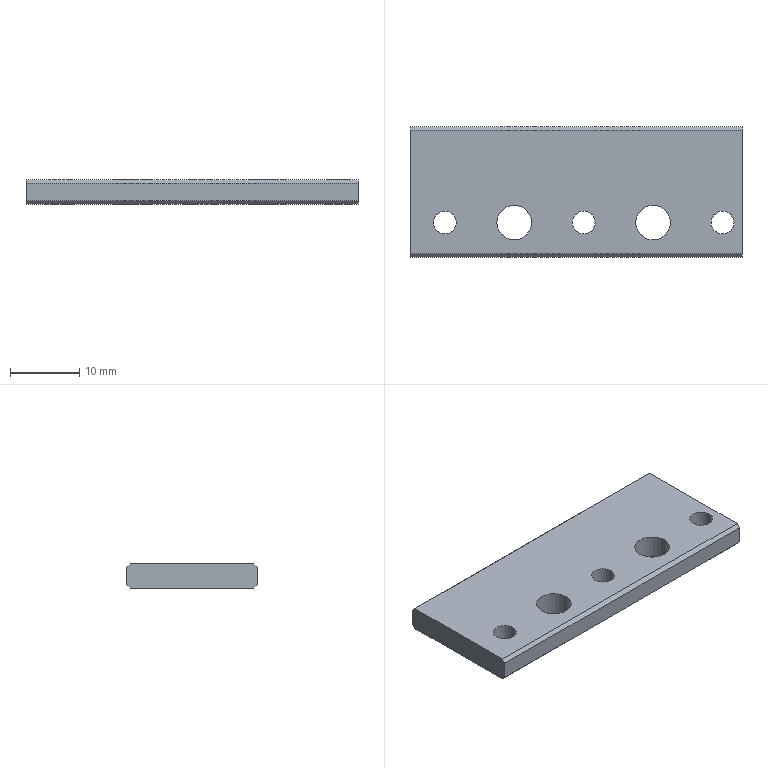Part | NX | 1 solid | 26 faces | box 47.8 x 18.8 x 3.5 mm | volume 2890 mm3 | plane 10 | cylinder 10 | cone 6 | commonest cylinder face diameters 3.3 x6 5 x4
STEP:
#1=CARTESIAN_POINT('',(4.5,18.3,0.));
#2=VERTEX_POINT('',#1);
#3=CARTESIAN_POINT('',(-43.3,18.3,0.));
#4=VERTEX_POINT('',#3);
#5=CARTESIAN_POINT('',(0.,18.3,0.));
#6=DIRECTION('',(-1.,0.,0.));
#7=VECTOR('',#6,1000.);
#8=LINE('',#5,#7);
#9=EDGE_CURVE('',#2,#4,#8,.T.);
#10=ORIENTED_EDGE('',*,*,#9,.T.);
#11=CARTESIAN_POINT('',(-43.3,0.5,0.));
#12=VERTEX_POINT('',#11);
#13=CARTESIAN_POINT('',(-43.3,0.,0.));
#14=DIRECTION('',(0.,1.,0.));
#15=VECTOR('',#14,1000.);
#16=LINE('',#13,#15);
#17=EDGE_CURVE('',#12,#4,#16,.T.);
#18=ORIENTED_EDGE('',*,*,#17,.F.);
#19=CARTESIAN_POINT('',(4.5,0.5,0.));
#20=VERTEX_POINT('',#19);
#21=CARTESIAN_POINT('',(0.,0.5,0.));
#22=DIRECTION('',(1.,0.,0.));
#23=VECTOR('',#22,1000.);
#24=LINE('',#21,#23);
#25=EDGE_CURVE('',#12,#20,#24,.T.);
#26=ORIENTED_EDGE('',*,*,#25,.T.);
#27=CARTESIAN_POINT('',(4.5,0.,0.));
#28=DIRECTION('',(0.,1.,0.));
#29=VECTOR('',#28,1000.);
#30=LINE('',#27,#29);
#31=EDGE_CURVE('',#20,#2,#30,.T.);
#32=ORIENTED_EDGE('',*,*,#31,.T.);
#33=EDGE_LOOP('',(#10,#18,#26,#32));
#34=FACE_BOUND('',#33,.T.);
#35=CARTESIAN_POINT('',(-39.95,5.,0.));
#36=VERTEX_POINT('',#35);
#37=CARTESIAN_POINT('',(-36.65,5.,0.));
#38=VERTEX_POINT('',#37);
#39=CARTESIAN_POINT('',(-38.3,5.,0.));
#40=DIRECTION('',(0.,0.,-1.));
#41=DIRECTION('',(-1.,0.,0.));
#42=AXIS2_PLACEMENT_3D('',#39,#40,#41);
#43=CIRCLE('',#42,1.65);
#44=EDGE_CURVE('',#36,#38,#43,.T.);
#45=ORIENTED_EDGE('',*,*,#44,.T.);
#46=CARTESIAN_POINT('',(-38.3,5.,0.));
#47=DIRECTION('',(0.,0.,-1.));
#48=DIRECTION('',(-1.,0.,0.));
#49=AXIS2_PLACEMENT_3D('',#46,#47,#48);
#50=CIRCLE('',#49,1.65);
#51=EDGE_CURVE('',#38,#36,#50,.T.);
#52=ORIENTED_EDGE('',*,*,#51,.T.);
#53=EDGE_LOOP('',(#45,#52));
#54=FACE_BOUND('',#53,.T.);
#55=CARTESIAN_POINT('',(-25.8,5.,0.));
#56=VERTEX_POINT('',#55);
#57=CARTESIAN_POINT('',(-30.8,5.,0.));
#58=VERTEX_POINT('',#57);
#59=CARTESIAN_POINT('',(-28.3,5.,0.));
#60=DIRECTION('',(0.,0.,1.));
#61=DIRECTION('',(1.,0.,0.));
#62=AXIS2_PLACEMENT_3D('',#59,#60,#61);
#63=CIRCLE('',#62,2.5);
#64=EDGE_CURVE('',#56,#58,#63,.T.);
#65=ORIENTED_EDGE('',*,*,#64,.F.);
#66=CARTESIAN_POINT('',(-28.3,5.,0.));
#67=DIRECTION('',(0.,0.,1.));
#68=DIRECTION('',(1.,0.,0.));
#69=AXIS2_PLACEMENT_3D('',#66,#67,#68);
#70=CIRCLE('',#69,2.5);
#71=EDGE_CURVE('',#58,#56,#70,.T.);
#72=ORIENTED_EDGE('',*,*,#71,.F.);
#73=EDGE_LOOP('',(#65,#72));
#74=FACE_BOUND('',#73,.T.);
#75=CARTESIAN_POINT('',(-10.8,5.,0.));
#76=VERTEX_POINT('',#75);
#77=CARTESIAN_POINT('',(-5.8,5.,0.));
#78=VERTEX_POINT('',#77);
#79=CARTESIAN_POINT('',(-8.3,5.,0.));
#80=DIRECTION('',(0.,0.,1.));
#81=DIRECTION('',(1.,0.,0.));
#82=AXIS2_PLACEMENT_3D('',#79,#80,#81);
#83=CIRCLE('',#82,2.5);
#84=EDGE_CURVE('',#76,#78,#83,.T.);
#85=ORIENTED_EDGE('',*,*,#84,.F.);
#86=CARTESIAN_POINT('',(-8.3,5.,0.));
#87=DIRECTION('',(0.,0.,1.));
#88=DIRECTION('',(1.,0.,0.));
#89=AXIS2_PLACEMENT_3D('',#86,#87,#88);
#90=CIRCLE('',#89,2.5);
#91=EDGE_CURVE('',#78,#76,#90,.T.);
#92=ORIENTED_EDGE('',*,*,#91,.F.);
#93=EDGE_LOOP('',(#85,#92));
#94=FACE_BOUND('',#93,.T.);
#95=CARTESIAN_POINT('',(0.05,5.,0.));
#96=VERTEX_POINT('',#95);
#97=CARTESIAN_POINT('',(3.35,5.,0.));
#98=VERTEX_POINT('',#97);
#99=CARTESIAN_POINT('',(1.7,5.,0.));
#100=DIRECTION('',(0.,0.,-1.));
#101=DIRECTION('',(-1.,0.,0.));
#102=AXIS2_PLACEMENT_3D('',#99,#100,#101);
#103=CIRCLE('',#102,1.65);
#104=EDGE_CURVE('',#96,#98,#103,.T.);
#105=ORIENTED_EDGE('',*,*,#104,.T.);
#106=CARTESIAN_POINT('',(1.7,5.,0.));
#107=DIRECTION('',(0.,0.,-1.));
#108=DIRECTION('',(-1.,0.,0.));
#109=AXIS2_PLACEMENT_3D('',#106,#107,#108);
#110=CIRCLE('',#109,1.65);
#111=EDGE_CURVE('',#98,#96,#110,.T.);
#112=ORIENTED_EDGE('',*,*,#111,.T.);
#113=EDGE_LOOP('',(#105,#112));
#114=FACE_BOUND('',#113,.T.);
#115=CARTESIAN_POINT('',(-19.95,5.,0.));
#116=VERTEX_POINT('',#115);
#117=CARTESIAN_POINT('',(-16.65,5.,0.));
#118=VERTEX_POINT('',#117);
#119=CARTESIAN_POINT('',(-18.3,5.,0.));
#120=DIRECTION('',(0.,0.,-1.));
#121=DIRECTION('',(-1.,0.,0.));
#122=AXIS2_PLACEMENT_3D('',#119,#120,#121);
#123=CIRCLE('',#122,1.65);
#124=EDGE_CURVE('',#116,#118,#123,.T.);
#125=ORIENTED_EDGE('',*,*,#124,.T.);
#126=CARTESIAN_POINT('',(-18.3,5.,0.));
#127=DIRECTION('',(0.,0.,-1.));
#128=DIRECTION('',(-1.,0.,0.));
#129=AXIS2_PLACEMENT_3D('',#126,#127,#128);
#130=CIRCLE('',#129,1.65);
#131=EDGE_CURVE('',#118,#116,#130,.T.);
#132=ORIENTED_EDGE('',*,*,#131,.T.);
#133=EDGE_LOOP('',(#125,#132));
#134=FACE_BOUND('',#133,.T.);
#135=CARTESIAN_POINT('',(0.,0.,0.));
#136=DIRECTION('',(0.,0.,1.));
#137=DIRECTION('',(1.,0.,0.));
#138=AXIS2_PLACEMENT_3D('',#135,#136,#137);
#139=PLANE('',#138);
#140=ADVANCED_FACE('',(#34,#54,#74,#94,#114,#134),#139,.T.);
#141=CARTESIAN_POINT('',(4.5,0.5,-3.5));
#142=VERTEX_POINT('',#141);
#143=CARTESIAN_POINT('',(4.5,18.3,-3.5));
#144=VERTEX_POINT('',#143);
#145=CARTESIAN_POINT('',(4.5,0.,-3.5));
#146=DIRECTION('',(0.,1.,0.));
#147=VECTOR('',#146,1000.);
#148=LINE('',#145,#147);
#149=EDGE_CURVE('',#142,#144,#148,.T.);
#150=ORIENTED_EDGE('',*,*,#149,.T.);
#151=CARTESIAN_POINT('',(4.5,18.8,-3.));
#152=VERTEX_POINT('',#151);
#153=CARTESIAN_POINT('',(4.5,21.8,0.));
#154=DIRECTION('',(0.,0.7071,0.7071));
#155=VECTOR('',#154,1000.);
#156=LINE('',#153,#155);
#157=EDGE_CURVE('',#144,#152,#156,.T.);
#158=ORIENTED_EDGE('',*,*,#157,.T.);
#159=CARTESIAN_POINT('',(4.5,18.8,-0.5));
#160=VERTEX_POINT('',#159);
#161=CARTESIAN_POINT('',(4.5,18.8,0.));
#162=DIRECTION('',(0.,0.,-1.));
#163=VECTOR('',#162,1000.);
#164=LINE('',#161,#163);
#165=EDGE_CURVE('',#160,#152,#164,.T.);
#166=ORIENTED_EDGE('',*,*,#165,.F.);
#167=CARTESIAN_POINT('',(4.5,18.3,0.));
#168=DIRECTION('',(0.,0.7071,-0.7071));
#169=VECTOR('',#168,1000.);
#170=LINE('',#167,#169);
#171=EDGE_CURVE('',#2,#160,#170,.T.);
#172=ORIENTED_EDGE('',*,*,#171,.F.);
#173=ORIENTED_EDGE('',*,*,#31,.F.);
#174=CARTESIAN_POINT('',(4.5,0.,-0.5));
#175=VERTEX_POINT('',#174);
#176=CARTESIAN_POINT('',(4.5,0.5,0.));
#177=DIRECTION('',(0.,0.7071,0.7071));
#178=VECTOR('',#177,1000.);
#179=LINE('',#176,#178);
#180=EDGE_CURVE('',#175,#20,#179,.T.);
#181=ORIENTED_EDGE('',*,*,#180,.F.);
#182=CARTESIAN_POINT('',(4.5,0.,-3.));
#183=VERTEX_POINT('',#182);
#184=CARTESIAN_POINT('',(4.5,0.,0.));
#185=DIRECTION('',(0.,0.,-1.));
#186=VECTOR('',#185,1000.);
#187=LINE('',#184,#186);
#188=EDGE_CURVE('',#175,#183,#187,.T.);
#189=ORIENTED_EDGE('',*,*,#188,.T.);
#190=CARTESIAN_POINT('',(4.5,-3.,0.));
#191=DIRECTION('',(0.,0.7071,-0.7071));
#192=VECTOR('',#191,1000.);
#193=LINE('',#190,#192);
#194=EDGE_CURVE('',#183,#142,#193,.T.);
#195=ORIENTED_EDGE('',*,*,#194,.T.);
#196=EDGE_LOOP('',(#150,#158,#166,#172,#173,#181,#189,#195));
#197=FACE_BOUND('',#196,.T.);
#198=CARTESIAN_POINT('',(4.5,18.8,0.));
#199=DIRECTION('',(-1.,0.,0.));
#200=DIRECTION('',(0.,0.,1.));
#201=AXIS2_PLACEMENT_3D('',#198,#199,#200);
#202=PLANE('',#201);
#203=ADVANCED_FACE('',(#197),#202,.F.);
#204=CARTESIAN_POINT('',(-43.3,18.3,-3.5));
#205=VERTEX_POINT('',#204);
#206=CARTESIAN_POINT('',(0.,18.3,-3.5));
#207=DIRECTION('',(1.,0.,0.));
#208=VECTOR('',#207,1000.);
#209=LINE('',#206,#208);
#210=EDGE_CURVE('',#205,#144,#209,.T.);
#211=ORIENTED_EDGE('',*,*,#210,.T.);
#212=ORIENTED_EDGE('',*,*,#149,.F.);
#213=CARTESIAN_POINT('',(-43.3,0.5,-3.5));
#214=VERTEX_POINT('',#213);
#215=CARTESIAN_POINT('',(0.,0.5,-3.5));
#216=DIRECTION('',(-1.,0.,0.));
#217=VECTOR('',#216,1000.);
#218=LINE('',#215,#217);
#219=EDGE_CURVE('',#142,#214,#218,.T.);
#220=ORIENTED_EDGE('',*,*,#219,.T.);
#221=CARTESIAN_POINT('',(-43.3,0.,-3.5));
#222=DIRECTION('',(0.,1.,0.));
#223=VECTOR('',#222,1000.);
#224=LINE('',#221,#223);
#225=EDGE_CURVE('',#214,#205,#224,.T.);
#226=ORIENTED_EDGE('',*,*,#225,.T.);
#227=EDGE_LOOP('',(#211,#212,#220,#226));
#228=FACE_BOUND('',#227,.T.);
#229=CARTESIAN_POINT('',(-40.615,5.,-3.5));
#230=VERTEX_POINT('',#229);
#231=CARTESIAN_POINT('',(-35.985,5.,-3.5));
#232=VERTEX_POINT('',#231);
#233=CARTESIAN_POINT('',(-38.3,5.,-3.5));
#234=DIRECTION('',(0.,0.,-1.));
#235=DIRECTION('',(-1.,0.,0.));
#236=AXIS2_PLACEMENT_3D('',#233,#234,#235);
#237=CIRCLE('',#236,2.315);
#238=EDGE_CURVE('',#230,#232,#237,.T.);
#239=ORIENTED_EDGE('',*,*,#238,.F.);
#240=CARTESIAN_POINT('',(-38.3,5.,-3.5));
#241=DIRECTION('',(0.,0.,-1.));
#242=DIRECTION('',(-1.,0.,0.));
#243=AXIS2_PLACEMENT_3D('',#240,#241,#242);
#244=CIRCLE('',#243,2.315);
#245=EDGE_CURVE('',#232,#230,#244,.T.);
#246=ORIENTED_EDGE('',*,*,#245,.F.);
#247=EDGE_LOOP('',(#239,#246));
#248=FACE_BOUND('',#247,.T.);
#249=CARTESIAN_POINT('',(-30.8,5.,-3.5));
#250=VERTEX_POINT('',#249);
#251=CARTESIAN_POINT('',(-25.8,5.,-3.5));
#252=VERTEX_POINT('',#251);
#253=CARTESIAN_POINT('',(-28.3,5.,-3.5));
#254=DIRECTION('',(0.,0.,1.));
#255=DIRECTION('',(1.,0.,0.));
#256=AXIS2_PLACEMENT_3D('',#253,#254,#255);
#257=CIRCLE('',#256,2.5);
#258=EDGE_CURVE('',#250,#252,#257,.T.);
#259=ORIENTED_EDGE('',*,*,#258,.T.);
#260=CARTESIAN_POINT('',(-28.3,5.,-3.5));
#261=DIRECTION('',(0.,0.,1.));
#262=DIRECTION('',(1.,0.,0.));
#263=AXIS2_PLACEMENT_3D('',#260,#261,#262);
#264=CIRCLE('',#263,2.5);
#265=EDGE_CURVE('',#252,#250,#264,.T.);
#266=ORIENTED_EDGE('',*,*,#265,.T.);
#267=EDGE_LOOP('',(#259,#266));
#268=FACE_BOUND('',#267,.T.);
#269=CARTESIAN_POINT('',(-5.8,5.,-3.5));
#270=VERTEX_POINT('',#269);
#271=CARTESIAN_POINT('',(-10.8,5.,-3.5));
#272=VERTEX_POINT('',#271);
#273=CARTESIAN_POINT('',(-8.3,5.,-3.5));
#274=DIRECTION('',(0.,0.,1.));
#275=DIRECTION('',(1.,0.,0.));
#276=AXIS2_PLACEMENT_3D('',#273,#274,#275);
#277=CIRCLE('',#276,2.5);
#278=EDGE_CURVE('',#270,#272,#277,.T.);
#279=ORIENTED_EDGE('',*,*,#278,.T.);
#280=CARTESIAN_POINT('',(-8.3,5.,-3.5));
#281=DIRECTION('',(0.,0.,1.));
#282=DIRECTION('',(1.,0.,0.));
#283=AXIS2_PLACEMENT_3D('',#280,#281,#282);
#284=CIRCLE('',#283,2.5);
#285=EDGE_CURVE('',#272,#270,#284,.T.);
#286=ORIENTED_EDGE('',*,*,#285,.T.);
#287=EDGE_LOOP('',(#279,#286));
#288=FACE_BOUND('',#287,.T.);
#289=CARTESIAN_POINT('',(-15.985,5.,-3.5));
#290=VERTEX_POINT('',#289);
#291=CARTESIAN_POINT('',(-20.615,5.,-3.5));
#292=VERTEX_POINT('',#291);
#293=CARTESIAN_POINT('',(-18.3,5.,-3.5));
#294=DIRECTION('',(0.,0.,-1.));
#295=DIRECTION('',(-1.,0.,0.));
#296=AXIS2_PLACEMENT_3D('',#293,#294,#295);
#297=CIRCLE('',#296,2.315);
#298=EDGE_CURVE('',#290,#292,#297,.T.);
#299=ORIENTED_EDGE('',*,*,#298,.F.);
#300=CARTESIAN_POINT('',(-18.3,5.,-3.5));
#301=DIRECTION('',(0.,0.,-1.));
#302=DIRECTION('',(-1.,0.,0.));
#303=AXIS2_PLACEMENT_3D('',#300,#301,#302);
#304=CIRCLE('',#303,2.315);
#305=EDGE_CURVE('',#292,#290,#304,.T.);
#306=ORIENTED_EDGE('',*,*,#305,.F.);
#307=EDGE_LOOP('',(#299,#306));
#308=FACE_BOUND('',#307,.T.);
#309=CARTESIAN_POINT('',(4.015,5.,-3.5));
#310=VERTEX_POINT('',#309);
#311=CARTESIAN_POINT('',(-0.615,5.,-3.5));
#312=VERTEX_POINT('',#311);
#313=CARTESIAN_POINT('',(1.7,5.,-3.5));
#314=DIRECTION('',(0.,0.,-1.));
#315=DIRECTION('',(-1.,0.,0.));
#316=AXIS2_PLACEMENT_3D('',#313,#314,#315);
#317=CIRCLE('',#316,2.315);
#318=EDGE_CURVE('',#310,#312,#317,.T.);
#319=ORIENTED_EDGE('',*,*,#318,.F.);
#320=CARTESIAN_POINT('',(1.7,5.,-3.5));
#321=DIRECTION('',(0.,0.,-1.));
#322=DIRECTION('',(-1.,0.,0.));
#323=AXIS2_PLACEMENT_3D('',#320,#321,#322);
#324=CIRCLE('',#323,2.315);
#325=EDGE_CURVE('',#312,#310,#324,.T.);
#326=ORIENTED_EDGE('',*,*,#325,.F.);
#327=EDGE_LOOP('',(#319,#326));
#328=FACE_BOUND('',#327,.T.);
#329=CARTESIAN_POINT('',(0.,0.,-3.5));
#330=DIRECTION('',(0.,0.,1.));
#331=DIRECTION('',(1.,0.,0.));
#332=AXIS2_PLACEMENT_3D('',#329,#330,#331);
#333=PLANE('',#332);
#334=ADVANCED_FACE('',(#228,#248,#268,#288,#308,#328),#333,.F.);
#335=CARTESIAN_POINT('',(-43.3,18.8,-3.));
#336=VERTEX_POINT('',#335);
#337=CARTESIAN_POINT('',(0.,18.8,-3.));
#338=DIRECTION('',(1.,0.,0.));
#339=VECTOR('',#338,1000.);
#340=LINE('',#337,#339);
#341=EDGE_CURVE('',#336,#152,#340,.T.);
#342=ORIENTED_EDGE('',*,*,#341,.F.);
#343=CARTESIAN_POINT('',(-43.3,18.8,-0.5));
#344=VERTEX_POINT('',#343);
#345=CARTESIAN_POINT('',(-43.3,18.8,-3.5));
#346=DIRECTION('',(0.,0.,1.));
#347=VECTOR('',#346,1000.);
#348=LINE('',#345,#347);
#349=EDGE_CURVE('',#336,#344,#348,.T.);
#350=ORIENTED_EDGE('',*,*,#349,.T.);
#351=CARTESIAN_POINT('',(0.,18.8,-0.5));
#352=DIRECTION('',(1.,0.,0.));
#353=VECTOR('',#352,1000.);
#354=LINE('',#351,#353);
#355=EDGE_CURVE('',#344,#160,#354,.T.);
#356=ORIENTED_EDGE('',*,*,#355,.T.);
#357=ORIENTED_EDGE('',*,*,#165,.T.);
#358=EDGE_LOOP('',(#342,#350,#356,#357));
#359=FACE_BOUND('',#358,.T.);
#360=CARTESIAN_POINT('',(8.,18.8,0.));
#361=DIRECTION('',(0.,1.,0.));
#362=DIRECTION('',(1.,0.,0.));
#363=AXIS2_PLACEMENT_3D('',#360,#361,#362);
#364=PLANE('',#363);
#365=ADVANCED_FACE('',(#359),#364,.T.);
#366=ORIENTED_EDGE('',*,*,#17,.T.);
#367=CARTESIAN_POINT('',(-43.3,18.3,0.));
#368=DIRECTION('',(0.,0.7071,-0.7071));
#369=VECTOR('',#368,1000.);
#370=LINE('',#367,#369);
#371=EDGE_CURVE('',#4,#344,#370,.T.);
#372=ORIENTED_EDGE('',*,*,#371,.T.);
#373=ORIENTED_EDGE('',*,*,#349,.F.);
#374=CARTESIAN_POINT('',(-43.3,21.8,0.));
#375=DIRECTION('',(0.,0.7071,0.7071));
#376=VECTOR('',#375,1000.);
#377=LINE('',#374,#376);
#378=EDGE_CURVE('',#205,#336,#377,.T.);
#379=ORIENTED_EDGE('',*,*,#378,.F.);
#380=ORIENTED_EDGE('',*,*,#225,.F.);
#381=CARTESIAN_POINT('',(-43.3,0.,-3.));
#382=VERTEX_POINT('',#381);
#383=CARTESIAN_POINT('',(-43.3,-3.,0.));
#384=DIRECTION('',(0.,0.7071,-0.7071));
#385=VECTOR('',#384,1000.);
#386=LINE('',#383,#385);
#387=EDGE_CURVE('',#382,#214,#386,.T.);
#388=ORIENTED_EDGE('',*,*,#387,.F.);
#389=CARTESIAN_POINT('',(-43.3,0.,-0.5));
#390=VERTEX_POINT('',#389);
#391=CARTESIAN_POINT('',(-43.3,0.,-3.5));
#392=DIRECTION('',(0.,0.,1.));
#393=VECTOR('',#392,1000.);
#394=LINE('',#391,#393);
#395=EDGE_CURVE('',#382,#390,#394,.T.);
#396=ORIENTED_EDGE('',*,*,#395,.T.);
#397=CARTESIAN_POINT('',(-43.3,0.5,0.));
#398=DIRECTION('',(0.,0.7071,0.7071));
#399=VECTOR('',#398,1000.);
#400=LINE('',#397,#399);
#401=EDGE_CURVE('',#390,#12,#400,.T.);
#402=ORIENTED_EDGE('',*,*,#401,.T.);
#403=EDGE_LOOP('',(#366,#372,#373,#379,#380,#388,#396,#402));
#404=FACE_BOUND('',#403,.T.);
#405=CARTESIAN_POINT('',(-43.3,18.8,0.));
#406=DIRECTION('',(-1.,0.,0.));
#407=DIRECTION('',(0.,0.,1.));
#408=AXIS2_PLACEMENT_3D('',#405,#406,#407);
#409=PLANE('',#408);
#410=ADVANCED_FACE('',(#404),#409,.T.);
#411=ORIENTED_EDGE('',*,*,#188,.F.);
#412=CARTESIAN_POINT('',(0.,0.,-0.5));
#413=DIRECTION('',(-1.,0.,0.));
#414=VECTOR('',#413,1000.);
#415=LINE('',#412,#414);
#416=EDGE_CURVE('',#175,#390,#415,.T.);
#417=ORIENTED_EDGE('',*,*,#416,.T.);
#418=ORIENTED_EDGE('',*,*,#395,.F.);
#419=CARTESIAN_POINT('',(0.,0.,-3.));
#420=DIRECTION('',(-1.,0.,0.));
#421=VECTOR('',#420,1000.);
#422=LINE('',#419,#421);
#423=EDGE_CURVE('',#183,#382,#422,.T.);
#424=ORIENTED_EDGE('',*,*,#423,.F.);
#425=EDGE_LOOP('',(#411,#417,#418,#424));
#426=FACE_BOUND('',#425,.T.);
#427=CARTESIAN_POINT('',(-43.3,0.,0.));
#428=DIRECTION('',(0.,-1.,0.));
#429=DIRECTION('',(0.,0.,-1.));
#430=AXIS2_PLACEMENT_3D('',#427,#428,#429);
#431=PLANE('',#430);
#432=ADVANCED_FACE('',(#426),#431,.T.);
#433=ORIENTED_EDGE('',*,*,#44,.F.);
#434=CARTESIAN_POINT('',(-39.95,5.,-3.116));
#435=VERTEX_POINT('',#434);
#436=CARTESIAN_POINT('',(-39.95,5.,-3.5));
#437=DIRECTION('',(0.,0.,-1.));
#438=VECTOR('',#437,1000.);
#439=LINE('',#436,#438);
#440=EDGE_CURVE('',#435,#36,#439,.F.);
#441=ORIENTED_EDGE('',*,*,#440,.F.);
#442=CARTESIAN_POINT('',(-36.65,5.,-3.116));
#443=VERTEX_POINT('',#442);
#444=CARTESIAN_POINT('',(-38.3,5.,-3.116));
#445=DIRECTION('',(0.,0.,-1.));
#446=DIRECTION('',(-1.,0.,0.));
#447=AXIS2_PLACEMENT_3D('',#444,#445,#446);
#448=CIRCLE('',#447,1.65);
#449=EDGE_CURVE('',#435,#443,#448,.T.);
#450=ORIENTED_EDGE('',*,*,#449,.T.);
#451=CARTESIAN_POINT('',(-36.65,5.,-3.5));
#452=DIRECTION('',(0.,0.,-1.));
#453=VECTOR('',#452,1000.);
#454=LINE('',#451,#453);
#455=EDGE_CURVE('',#443,#38,#454,.F.);
#456=ORIENTED_EDGE('',*,*,#455,.T.);
#457=EDGE_LOOP('',(#433,#441,#450,#456));
#458=FACE_BOUND('',#457,.T.);
#459=CARTESIAN_POINT('',(-38.3,5.,-3.5));
#460=DIRECTION('',(0.,0.,-1.));
#461=DIRECTION('',(-1.,0.,0.));
#462=AXIS2_PLACEMENT_3D('',#459,#460,#461);
#463=CYLINDRICAL_SURFACE('',#462,1.65);
#464=ADVANCED_FACE('',(#458),#463,.F.);
#465=ORIENTED_EDGE('',*,*,#238,.T.);
#466=CARTESIAN_POINT('',(-36.65,5.,-3.116));
#467=DIRECTION('',(0.866,0.,-0.5));
#468=VECTOR('',#467,1000.);
#469=LINE('',#466,#468);
#470=EDGE_CURVE('',#443,#232,#469,.T.);
#471=ORIENTED_EDGE('',*,*,#470,.F.);
#472=ORIENTED_EDGE('',*,*,#449,.F.);
#473=CARTESIAN_POINT('',(-39.95,5.,-3.116));
#474=DIRECTION('',(-0.866,0.,-0.5));
#475=VECTOR('',#474,1000.);
#476=LINE('',#473,#475);
#477=EDGE_CURVE('',#435,#230,#476,.T.);
#478=ORIENTED_EDGE('',*,*,#477,.T.);
#479=EDGE_LOOP('',(#465,#471,#472,#478));
#480=FACE_BOUND('',#479,.T.);
#481=CARTESIAN_POINT('',(-38.3,5.,-3.116));
#482=DIRECTION('',(0.,0.,-1.));
#483=DIRECTION('',(-1.,0.,0.));
#484=AXIS2_PLACEMENT_3D('',#481,#482,#483);
#485=CONICAL_SURFACE('',#484,1.65,1.047);
#486=ADVANCED_FACE('',(#480),#485,.F.);
#487=ORIENTED_EDGE('',*,*,#124,.F.);
#488=CARTESIAN_POINT('',(-19.95,5.,-3.116));
#489=VERTEX_POINT('',#488);
#490=CARTESIAN_POINT('',(-19.95,5.,-3.5));
#491=DIRECTION('',(0.,0.,-1.));
#492=VECTOR('',#491,1000.);
#493=LINE('',#490,#492);
#494=EDGE_CURVE('',#489,#116,#493,.F.);
#495=ORIENTED_EDGE('',*,*,#494,.F.);
#496=CARTESIAN_POINT('',(-16.65,5.,-3.116));
#497=VERTEX_POINT('',#496);
#498=CARTESIAN_POINT('',(-18.3,5.,-3.116));
#499=DIRECTION('',(0.,0.,-1.));
#500=DIRECTION('',(-1.,0.,0.));
#501=AXIS2_PLACEMENT_3D('',#498,#499,#500);
#502=CIRCLE('',#501,1.65);
#503=EDGE_CURVE('',#489,#497,#502,.T.);
#504=ORIENTED_EDGE('',*,*,#503,.T.);
#505=CARTESIAN_POINT('',(-16.65,5.,-3.5));
#506=DIRECTION('',(0.,0.,-1.));
#507=VECTOR('',#506,1000.);
#508=LINE('',#505,#507);
#509=EDGE_CURVE('',#497,#118,#508,.F.);
#510=ORIENTED_EDGE('',*,*,#509,.T.);
#511=EDGE_LOOP('',(#487,#495,#504,#510));
#512=FACE_BOUND('',#511,.T.);
#513=CARTESIAN_POINT('',(-18.3,5.,-3.5));
#514=DIRECTION('',(0.,0.,-1.));
#515=DIRECTION('',(-1.,0.,0.));
#516=AXIS2_PLACEMENT_3D('',#513,#514,#515);
#517=CYLINDRICAL_SURFACE('',#516,1.65);
#518=ADVANCED_FACE('',(#512),#517,.F.);
#519=ORIENTED_EDGE('',*,*,#298,.T.);
#520=CARTESIAN_POINT('',(-19.95,5.,-3.116));
#521=DIRECTION('',(-0.866,0.,-0.5));
#522=VECTOR('',#521,1000.);
#523=LINE('',#520,#522);
#524=EDGE_CURVE('',#292,#489,#523,.F.);
#525=ORIENTED_EDGE('',*,*,#524,.T.);
#526=CARTESIAN_POINT('',(-18.3,5.,-3.116));
#527=DIRECTION('',(0.,0.,-1.));
#528=DIRECTION('',(-1.,0.,0.));
#529=AXIS2_PLACEMENT_3D('',#526,#527,#528);
#530=CIRCLE('',#529,1.65);
#531=EDGE_CURVE('',#497,#489,#530,.T.);
#532=ORIENTED_EDGE('',*,*,#531,.F.);
#533=CARTESIAN_POINT('',(-16.65,5.,-3.116));
#534=DIRECTION('',(0.866,0.,-0.5));
#535=VECTOR('',#534,1000.);
#536=LINE('',#533,#535);
#537=EDGE_CURVE('',#290,#497,#536,.F.);
#538=ORIENTED_EDGE('',*,*,#537,.F.);
#539=EDGE_LOOP('',(#519,#525,#532,#538));
#540=FACE_BOUND('',#539,.T.);
#541=CARTESIAN_POINT('',(-18.3,5.,-3.116));
#542=DIRECTION('',(0.,0.,-1.));
#543=DIRECTION('',(-1.,0.,0.));
#544=AXIS2_PLACEMENT_3D('',#541,#542,#543);
#545=CONICAL_SURFACE('',#544,1.65,1.047);
#546=ADVANCED_FACE('',(#540),#545,.F.);
#547=CARTESIAN_POINT('',(3.35,5.,-3.116));
#548=VERTEX_POINT('',#547);
#549=CARTESIAN_POINT('',(0.05,5.,-3.116));
#550=VERTEX_POINT('',#549);
#551=CARTESIAN_POINT('',(1.7,5.,-3.116));
#552=DIRECTION('',(0.,0.,-1.));
#553=DIRECTION('',(-1.,0.,0.));
#554=AXIS2_PLACEMENT_3D('',#551,#552,#553);
#555=CIRCLE('',#554,1.65);
#556=EDGE_CURVE('',#548,#550,#555,.T.);
#557=ORIENTED_EDGE('',*,*,#556,.T.);
#558=CARTESIAN_POINT('',(0.05,5.,-3.5));
#559=DIRECTION('',(0.,0.,-1.));
#560=VECTOR('',#559,1000.);
#561=LINE('',#558,#560);
#562=EDGE_CURVE('',#550,#96,#561,.F.);
#563=ORIENTED_EDGE('',*,*,#562,.T.);
#564=ORIENTED_EDGE('',*,*,#111,.F.);
#565=CARTESIAN_POINT('',(3.35,5.,-3.5));
#566=DIRECTION('',(0.,0.,-1.));
#567=VECTOR('',#566,1000.);
#568=LINE('',#565,#567);
#569=EDGE_CURVE('',#548,#98,#568,.F.);
#570=ORIENTED_EDGE('',*,*,#569,.F.);
#571=EDGE_LOOP('',(#557,#563,#564,#570));
#572=FACE_BOUND('',#571,.T.);
#573=CARTESIAN_POINT('',(1.7,5.,-3.5));
#574=DIRECTION('',(0.,0.,-1.));
#575=DIRECTION('',(-1.,0.,0.));
#576=AXIS2_PLACEMENT_3D('',#573,#574,#575);
#577=CYLINDRICAL_SURFACE('',#576,1.65);
#578=ADVANCED_FACE('',(#572),#577,.F.);
#579=ORIENTED_EDGE('',*,*,#556,.F.);
#580=CARTESIAN_POINT('',(3.35,5.,-3.116));
#581=DIRECTION('',(0.866,0.,-0.5));
#582=VECTOR('',#581,1000.);
#583=LINE('',#580,#582);
#584=EDGE_CURVE('',#310,#548,#583,.F.);
#585=ORIENTED_EDGE('',*,*,#584,.F.);
#586=ORIENTED_EDGE('',*,*,#318,.T.);
#587=CARTESIAN_POINT('',(0.05,5.,-3.116));
#588=DIRECTION('',(-0.866,0.,-0.5));
#589=VECTOR('',#588,1000.);
#590=LINE('',#587,#589);
#591=EDGE_CURVE('',#312,#550,#590,.F.);
#592=ORIENTED_EDGE('',*,*,#591,.T.);
#593=EDGE_LOOP('',(#579,#585,#586,#592));
#594=FACE_BOUND('',#593,.T.);
#595=CARTESIAN_POINT('',(1.7,5.,-3.116));
#596=DIRECTION('',(0.,0.,-1.));
#597=DIRECTION('',(-1.,0.,0.));
#598=AXIS2_PLACEMENT_3D('',#595,#596,#597);
#599=CONICAL_SURFACE('',#598,1.65,1.047);
#600=ADVANCED_FACE('',(#594),#599,.F.);
#601=ORIENTED_EDGE('',*,*,#278,.F.);
#602=CARTESIAN_POINT('',(-5.8,5.,-3.85));
#603=DIRECTION('',(0.,0.,1.));
#604=VECTOR('',#603,1000.);
#605=LINE('',#602,#604);
#606=EDGE_CURVE('',#270,#78,#605,.T.);
#607=ORIENTED_EDGE('',*,*,#606,.T.);
#608=ORIENTED_EDGE('',*,*,#91,.T.);
#609=CARTESIAN_POINT('',(-10.8,5.,-3.85));
#610=DIRECTION('',(0.,0.,1.));
#611=VECTOR('',#610,1000.);
#612=LINE('',#609,#611);
#613=EDGE_CURVE('',#272,#76,#612,.T.);
#614=ORIENTED_EDGE('',*,*,#613,.F.);
#615=EDGE_LOOP('',(#601,#607,#608,#614));
#616=FACE_BOUND('',#615,.T.);
#617=CARTESIAN_POINT('',(-8.3,5.,-3.85));
#618=DIRECTION('',(0.,0.,1.));
#619=DIRECTION('',(1.,0.,0.));
#620=AXIS2_PLACEMENT_3D('',#617,#618,#619);
#621=CYLINDRICAL_SURFACE('',#620,2.5);
#622=ADVANCED_FACE('',(#616),#621,.F.);
#623=ORIENTED_EDGE('',*,*,#258,.F.);
#624=CARTESIAN_POINT('',(-30.8,5.,-3.85));
#625=DIRECTION('',(0.,0.,1.));
#626=VECTOR('',#625,1000.);
#627=LINE('',#624,#626);
#628=EDGE_CURVE('',#58,#250,#627,.F.);
#629=ORIENTED_EDGE('',*,*,#628,.F.);
#630=ORIENTED_EDGE('',*,*,#71,.T.);
#631=CARTESIAN_POINT('',(-25.8,5.,-3.85));
#632=DIRECTION('',(0.,0.,1.));
#633=VECTOR('',#632,1000.);
#634=LINE('',#631,#633);
#635=EDGE_CURVE('',#56,#252,#634,.F.);
#636=ORIENTED_EDGE('',*,*,#635,.T.);
#637=EDGE_LOOP('',(#623,#629,#630,#636));
#638=FACE_BOUND('',#637,.T.);
#639=CARTESIAN_POINT('',(-28.3,5.,-3.85));
#640=DIRECTION('',(0.,0.,1.));
#641=DIRECTION('',(1.,0.,0.));
#642=AXIS2_PLACEMENT_3D('',#639,#640,#641);
#643=CYLINDRICAL_SURFACE('',#642,2.5);
#644=ADVANCED_FACE('',(#638),#643,.F.);
#645=ORIENTED_EDGE('',*,*,#25,.F.);
#646=ORIENTED_EDGE('',*,*,#401,.F.);
#647=ORIENTED_EDGE('',*,*,#416,.F.);
#648=ORIENTED_EDGE('',*,*,#180,.T.);
#649=EDGE_LOOP('',(#645,#646,#647,#648));
#650=FACE_BOUND('',#649,.T.);
#651=CARTESIAN_POINT('',(-19.4,0.25,-0.25));
#652=DIRECTION('',(0.,0.7071,-0.7071));
#653=DIRECTION('',(-1.,0.,0.));
#654=AXIS2_PLACEMENT_3D('',#651,#652,#653);
#655=PLANE('',#654);
#656=ADVANCED_FACE('',(#650),#655,.F.);
#657=ORIENTED_EDGE('',*,*,#219,.F.);
#658=ORIENTED_EDGE('',*,*,#194,.F.);
#659=ORIENTED_EDGE('',*,*,#423,.T.);
#660=ORIENTED_EDGE('',*,*,#387,.T.);
#661=EDGE_LOOP('',(#657,#658,#659,#660));
#662=FACE_BOUND('',#661,.T.);
#663=CARTESIAN_POINT('',(-19.4,0.25,-3.25));
#664=DIRECTION('',(0.,-0.7071,-0.7071));
#665=DIRECTION('',(0.,-0.7071,0.7071));
#666=AXIS2_PLACEMENT_3D('',#663,#664,#665);
#667=PLANE('',#666);
#668=ADVANCED_FACE('',(#662),#667,.T.);
#669=ORIENTED_EDGE('',*,*,#9,.F.);
#670=ORIENTED_EDGE('',*,*,#171,.T.);
#671=ORIENTED_EDGE('',*,*,#355,.F.);
#672=ORIENTED_EDGE('',*,*,#371,.F.);
#673=EDGE_LOOP('',(#669,#670,#671,#672));
#674=FACE_BOUND('',#673,.T.);
#675=CARTESIAN_POINT('',(-19.4,18.55,-0.25));
#676=DIRECTION('',(0.,-0.7071,-0.7071));
#677=DIRECTION('',(0.,-0.7071,0.7071));
#678=AXIS2_PLACEMENT_3D('',#675,#676,#677);
#679=PLANE('',#678);
#680=ADVANCED_FACE('',(#674),#679,.F.);
#681=ORIENTED_EDGE('',*,*,#210,.F.);
#682=ORIENTED_EDGE('',*,*,#378,.T.);
#683=ORIENTED_EDGE('',*,*,#341,.T.);
#684=ORIENTED_EDGE('',*,*,#157,.F.);
#685=EDGE_LOOP('',(#681,#682,#683,#684));
#686=FACE_BOUND('',#685,.T.);
#687=CARTESIAN_POINT('',(-19.4,18.55,-3.25));
#688=DIRECTION('',(0.,0.7071,-0.7071));
#689=DIRECTION('',(-1.,0.,0.));
#690=AXIS2_PLACEMENT_3D('',#687,#688,#689);
#691=PLANE('',#690);
#692=ADVANCED_FACE('',(#686),#691,.T.);
#693=ORIENTED_EDGE('',*,*,#84,.T.);
#694=ORIENTED_EDGE('',*,*,#606,.F.);
#695=ORIENTED_EDGE('',*,*,#285,.F.);
#696=ORIENTED_EDGE('',*,*,#613,.T.);
#697=EDGE_LOOP('',(#693,#694,#695,#696));
#698=FACE_BOUND('',#697,.T.);
#699=CARTESIAN_POINT('',(-8.3,5.,-3.85));
#700=DIRECTION('',(0.,0.,1.));
#701=DIRECTION('',(1.,0.,0.));
#702=AXIS2_PLACEMENT_3D('',#699,#700,#701);
#703=CYLINDRICAL_SURFACE('',#702,2.5);
#704=ADVANCED_FACE('',(#698),#703,.F.);
#705=ORIENTED_EDGE('',*,*,#470,.T.);
#706=ORIENTED_EDGE('',*,*,#245,.T.);
#707=ORIENTED_EDGE('',*,*,#477,.F.);
#708=CARTESIAN_POINT('',(-38.3,5.,-3.116));
#709=DIRECTION('',(0.,0.,-1.));
#710=DIRECTION('',(-1.,0.,0.));
#711=AXIS2_PLACEMENT_3D('',#708,#709,#710);
#712=CIRCLE('',#711,1.65);
#713=EDGE_CURVE('',#443,#435,#712,.T.);
#714=ORIENTED_EDGE('',*,*,#713,.F.);
#715=EDGE_LOOP('',(#705,#706,#707,#714));
#716=FACE_BOUND('',#715,.T.);
#717=CARTESIAN_POINT('',(-38.3,5.,-3.116));
#718=DIRECTION('',(0.,0.,-1.));
#719=DIRECTION('',(-1.,0.,0.));
#720=AXIS2_PLACEMENT_3D('',#717,#718,#719);
#721=CONICAL_SURFACE('',#720,1.65,1.047);
#722=ADVANCED_FACE('',(#716),#721,.F.);
#723=ORIENTED_EDGE('',*,*,#104,.F.);
#724=ORIENTED_EDGE('',*,*,#562,.F.);
#725=CARTESIAN_POINT('',(1.7,5.,-3.116));
#726=DIRECTION('',(0.,0.,-1.));
#727=DIRECTION('',(-1.,0.,0.));
#728=AXIS2_PLACEMENT_3D('',#725,#726,#727);
#729=CIRCLE('',#728,1.65);
#730=EDGE_CURVE('',#550,#548,#729,.T.);
#731=ORIENTED_EDGE('',*,*,#730,.T.);
#732=ORIENTED_EDGE('',*,*,#569,.T.);
#733=EDGE_LOOP('',(#723,#724,#731,#732));
#734=FACE_BOUND('',#733,.T.);
#735=CARTESIAN_POINT('',(1.7,5.,-3.5));
#736=DIRECTION('',(0.,0.,-1.));
#737=DIRECTION('',(-1.,0.,0.));
#738=AXIS2_PLACEMENT_3D('',#735,#736,#737);
#739=CYLINDRICAL_SURFACE('',#738,1.65);
#740=ADVANCED_FACE('',(#734),#739,.F.);
#741=ORIENTED_EDGE('',*,*,#503,.F.);
#742=ORIENTED_EDGE('',*,*,#524,.F.);
#743=ORIENTED_EDGE('',*,*,#305,.T.);
#744=ORIENTED_EDGE('',*,*,#537,.T.);
#745=EDGE_LOOP('',(#741,#742,#743,#744));
#746=FACE_BOUND('',#745,.T.);
#747=CARTESIAN_POINT('',(-18.3,5.,-3.116));
#748=DIRECTION('',(0.,0.,-1.));
#749=DIRECTION('',(-1.,0.,0.));
#750=AXIS2_PLACEMENT_3D('',#747,#748,#749);
#751=CONICAL_SURFACE('',#750,1.65,1.047);
#752=ADVANCED_FACE('',(#746),#751,.F.);
#753=ORIENTED_EDGE('',*,*,#440,.T.);
#754=ORIENTED_EDGE('',*,*,#51,.F.);
#755=ORIENTED_EDGE('',*,*,#455,.F.);
#756=ORIENTED_EDGE('',*,*,#713,.T.);
#757=EDGE_LOOP('',(#753,#754,#755,#756));
#758=FACE_BOUND('',#757,.T.);
#759=CARTESIAN_POINT('',(-38.3,5.,-3.5));
#760=DIRECTION('',(0.,0.,-1.));
#761=DIRECTION('',(-1.,0.,0.));
#762=AXIS2_PLACEMENT_3D('',#759,#760,#761);
#763=CYLINDRICAL_SURFACE('',#762,1.65);
#764=ADVANCED_FACE('',(#758),#763,.F.);
#765=ORIENTED_EDGE('',*,*,#494,.T.);
#766=ORIENTED_EDGE('',*,*,#131,.F.);
#767=ORIENTED_EDGE('',*,*,#509,.F.);
#768=ORIENTED_EDGE('',*,*,#531,.T.);
#769=EDGE_LOOP('',(#765,#766,#767,#768));
#770=FACE_BOUND('',#769,.T.);
#771=CARTESIAN_POINT('',(-18.3,5.,-3.5));
#772=DIRECTION('',(0.,0.,-1.));
#773=DIRECTION('',(-1.,0.,0.));
#774=AXIS2_PLACEMENT_3D('',#771,#772,#773);
#775=CYLINDRICAL_SURFACE('',#774,1.65);
#776=ADVANCED_FACE('',(#770),#775,.F.);
#777=ORIENTED_EDGE('',*,*,#64,.T.);
#778=ORIENTED_EDGE('',*,*,#628,.T.);
#779=ORIENTED_EDGE('',*,*,#265,.F.);
#780=ORIENTED_EDGE('',*,*,#635,.F.);
#781=EDGE_LOOP('',(#777,#778,#779,#780));
#782=FACE_BOUND('',#781,.T.);
#783=CARTESIAN_POINT('',(-28.3,5.,-3.85));
#784=DIRECTION('',(0.,0.,1.));
#785=DIRECTION('',(1.,0.,0.));
#786=AXIS2_PLACEMENT_3D('',#783,#784,#785);
#787=CYLINDRICAL_SURFACE('',#786,2.5);
#788=ADVANCED_FACE('',(#782),#787,.F.);
#789=ORIENTED_EDGE('',*,*,#591,.F.);
#790=ORIENTED_EDGE('',*,*,#325,.T.);
#791=ORIENTED_EDGE('',*,*,#584,.T.);
#792=ORIENTED_EDGE('',*,*,#730,.F.);
#793=EDGE_LOOP('',(#789,#790,#791,#792));
#794=FACE_BOUND('',#793,.T.);
#795=CARTESIAN_POINT('',(1.7,5.,-3.116));
#796=DIRECTION('',(0.,0.,-1.));
#797=DIRECTION('',(-1.,0.,0.));
#798=AXIS2_PLACEMENT_3D('',#795,#796,#797);
#799=CONICAL_SURFACE('',#798,1.65,1.047);
#800=ADVANCED_FACE('',(#794),#799,.F.);
#801=CLOSED_SHELL('',(#140,#203,#334,#365,#410,#432,#464,#486,#518,#546,#578,#600,#622,#644,#656,#668,#680,#692,#704,#722,#740,#752,#764,#776,#788,#800));
#802=MANIFOLD_SOLID_BREP('',#801);
#803=(LENGTH_UNIT()NAMED_UNIT(*)SI_UNIT(.MILLI.,.METRE.));
#804=UNCERTAINTY_MEASURE_WITH_UNIT(LENGTH_MEASURE(0.00001),#803,'','');
#805=(NAMED_UNIT(*)PLANE_ANGLE_UNIT()SI_UNIT($,.RADIAN.));
#806=(NAMED_UNIT(*)SI_UNIT($,.STERADIAN.)SOLID_ANGLE_UNIT());
#807=(GEOMETRIC_REPRESENTATION_CONTEXT(3)GLOBAL_UNCERTAINTY_ASSIGNED_CONTEXT((#804))GLOBAL_UNIT_ASSIGNED_CONTEXT((#803,#805,#806))REPRESENTATION_CONTEXT('',''));
#808=ADVANCED_BREP_SHAPE_REPRESENTATION('',(#802),#807);